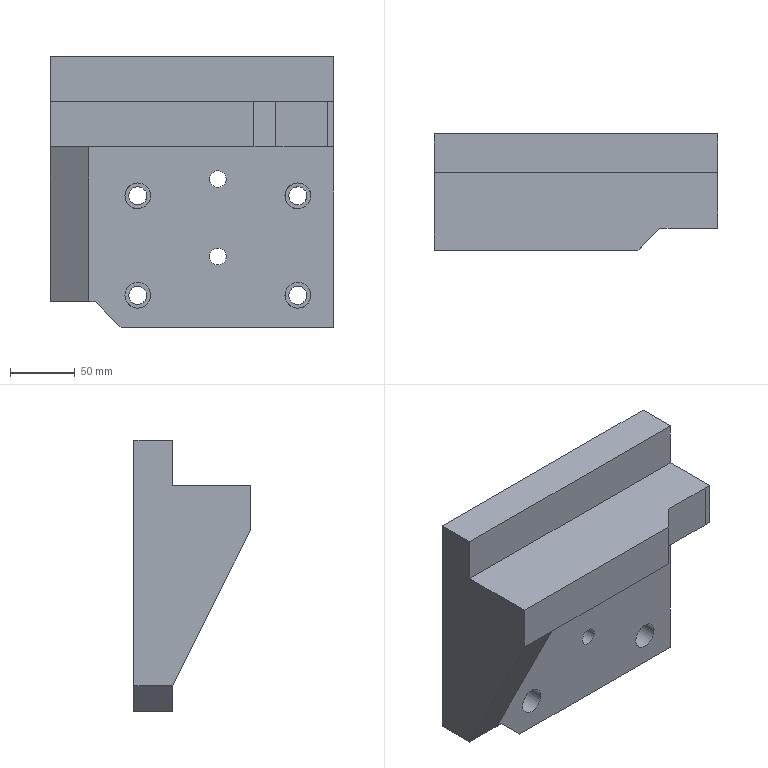Part | NX | features solid 2 | 1 solid | 31 faces | box 220 x 90 x 210 mm | volume 1861118 mm3 | plane 21 | cylinder 10 | commonest cylinder face diameters 14 x4 20 x4 13 x2
STEP:
#1=CARTESIAN_POINT('',(248.,505.,-125.));
#2=VERTEX_POINT('',#1);
#3=CARTESIAN_POINT('',(120.,505.,-125.));
#4=VERTEX_POINT('',#3);
#5=CARTESIAN_POINT('',(-235.,505.,-125.));
#6=DIRECTION('',(-1.,0.,0.));
#7=VECTOR('',#6,1000.);
#8=LINE('',#5,#7);
#9=EDGE_CURVE('',#2,#4,#8,.T.);
#10=ORIENTED_EDGE('',*,*,#9,.T.);
#11=CARTESIAN_POINT('',(120.,565.,-125.));
#12=VERTEX_POINT('',#11);
#13=CARTESIAN_POINT('',(120.,565.,-125.));
#14=DIRECTION('',(0.,1.,0.));
#15=VECTOR('',#14,1000.);
#16=LINE('',#13,#15);
#17=EDGE_CURVE('',#12,#4,#16,.F.);
#18=ORIENTED_EDGE('',*,*,#17,.F.);
#19=CARTESIAN_POINT('',(310.,565.,-125.));
#20=VERTEX_POINT('',#19);
#21=CARTESIAN_POINT('',(-235.,565.,-125.));
#22=DIRECTION('',(1.,0.,0.));
#23=VECTOR('',#22,1000.);
#24=LINE('',#21,#23);
#25=EDGE_CURVE('',#12,#20,#24,.T.);
#26=ORIENTED_EDGE('',*,*,#25,.T.);
#27=CARTESIAN_POINT('',(310.,522.,-125.));
#28=VERTEX_POINT('',#27);
#29=CARTESIAN_POINT('',(310.,565.,-125.));
#30=DIRECTION('',(0.,1.,0.));
#31=VECTOR('',#30,1000.);
#32=LINE('',#29,#31);
#33=EDGE_CURVE('',#20,#28,#32,.F.);
#34=ORIENTED_EDGE('',*,*,#33,.T.);
#35=CARTESIAN_POINT('',(305.,522.,-125.));
#36=VERTEX_POINT('',#35);
#37=CARTESIAN_POINT('',(-235.,522.,-125.));
#38=DIRECTION('',(1.,0.,0.));
#39=VECTOR('',#38,1000.);
#40=LINE('',#37,#39);
#41=EDGE_CURVE('',#28,#36,#40,.F.);
#42=ORIENTED_EDGE('',*,*,#41,.T.);
#43=CARTESIAN_POINT('',(265.,522.,-125.));
#44=VERTEX_POINT('',#43);
#45=CARTESIAN_POINT('',(-235.,522.,-125.));
#46=DIRECTION('',(1.,0.,0.));
#47=VECTOR('',#46,1000.);
#48=LINE('',#45,#47);
#49=EDGE_CURVE('',#44,#36,#48,.T.);
#50=ORIENTED_EDGE('',*,*,#49,.F.);
#51=CARTESIAN_POINT('',(36.5,293.5,-125.));
#52=DIRECTION('',(-0.7071,-0.7071,0.));
#53=VECTOR('',#52,1000.);
#54=LINE('',#51,#53);
#55=EDGE_CURVE('',#44,#2,#54,.T.);
#56=ORIENTED_EDGE('',*,*,#55,.T.);
#57=EDGE_LOOP('',(#10,#18,#26,#34,#42,#50,#56));
#58=FACE_BOUND('',#57,.T.);
#59=CARTESIAN_POINT('',(-235.,565.,-125.));
#60=DIRECTION('',(0.,0.,1.));
#61=DIRECTION('',(1.,0.,0.));
#62=AXIS2_PLACEMENT_3D('',#59,#60,#61);
#63=PLANE('',#62);
#64=ADVANCED_FACE('',(#58),#63,.F.);
#65=CARTESIAN_POINT('',(148.,565.,-163.));
#66=VERTEX_POINT('',#65);
#67=CARTESIAN_POINT('',(158.,565.,-163.));
#68=DIRECTION('',(0.,1.,0.));
#69=DIRECTION('',(-1.,0.,0.));
#70=AXIS2_PLACEMENT_3D('',#67,#68,#69);
#71=CIRCLE('',#70,10.);
#72=EDGE_CURVE('',#66,#66,#71,.F.);
#73=ORIENTED_EDGE('',*,*,#72,.F.);
#74=EDGE_LOOP('',(#73));
#75=FACE_BOUND('',#74,.T.);
#76=CARTESIAN_POINT('',(272.,565.,-163.));
#77=VERTEX_POINT('',#76);
#78=CARTESIAN_POINT('',(282.,565.,-163.));
#79=DIRECTION('',(0.,1.,0.));
#80=DIRECTION('',(-1.,0.,0.));
#81=AXIS2_PLACEMENT_3D('',#78,#79,#80);
#82=CIRCLE('',#81,10.);
#83=EDGE_CURVE('',#77,#77,#82,.F.);
#84=ORIENTED_EDGE('',*,*,#83,.F.);
#85=EDGE_LOOP('',(#84));
#86=FACE_BOUND('',#85,.T.);
#87=CARTESIAN_POINT('',(213.5,565.,-150.));
#88=VERTEX_POINT('',#87);
#89=CARTESIAN_POINT('',(220.,565.,-150.));
#90=DIRECTION('',(0.,1.,0.));
#91=DIRECTION('',(-1.,0.,0.));
#92=AXIS2_PLACEMENT_3D('',#89,#90,#91);
#93=CIRCLE('',#92,6.5);
#94=EDGE_CURVE('',#88,#88,#93,.T.);
#95=ORIENTED_EDGE('',*,*,#94,.T.);
#96=EDGE_LOOP('',(#95));
#97=FACE_BOUND('',#96,.T.);
#98=CARTESIAN_POINT('',(213.5,565.,-210.));
#99=VERTEX_POINT('',#98);
#100=CARTESIAN_POINT('',(220.,565.,-210.));
#101=DIRECTION('',(0.,1.,0.));
#102=DIRECTION('',(-1.,0.,0.));
#103=AXIS2_PLACEMENT_3D('',#100,#101,#102);
#104=CIRCLE('',#103,6.5);
#105=EDGE_CURVE('',#99,#99,#104,.T.);
#106=ORIENTED_EDGE('',*,*,#105,.T.);
#107=EDGE_LOOP('',(#106));
#108=FACE_BOUND('',#107,.T.);
#109=CARTESIAN_POINT('',(148.,565.,-240.));
#110=VERTEX_POINT('',#109);
#111=CARTESIAN_POINT('',(158.,565.,-240.));
#112=DIRECTION('',(0.,1.,0.));
#113=DIRECTION('',(-1.,0.,0.));
#114=AXIS2_PLACEMENT_3D('',#111,#112,#113);
#115=CIRCLE('',#114,10.);
#116=EDGE_CURVE('',#110,#110,#115,.F.);
#117=ORIENTED_EDGE('',*,*,#116,.F.);
#118=EDGE_LOOP('',(#117));
#119=FACE_BOUND('',#118,.T.);
#120=CARTESIAN_POINT('',(272.,565.,-240.));
#121=VERTEX_POINT('',#120);
#122=CARTESIAN_POINT('',(282.,565.,-240.));
#123=DIRECTION('',(0.,1.,0.));
#124=DIRECTION('',(-1.,0.,0.));
#125=AXIS2_PLACEMENT_3D('',#122,#123,#124);
#126=CIRCLE('',#125,10.);
#127=EDGE_CURVE('',#121,#121,#126,.F.);
#128=ORIENTED_EDGE('',*,*,#127,.F.);
#129=EDGE_LOOP('',(#128));
#130=FACE_BOUND('',#129,.T.);
#131=ORIENTED_EDGE('',*,*,#25,.F.);
#132=CARTESIAN_POINT('',(120.,565.,-245.));
#133=VERTEX_POINT('',#132);
#134=CARTESIAN_POINT('',(120.,565.,-125.));
#135=DIRECTION('',(0.,0.,-1.));
#136=VECTOR('',#135,1000.);
#137=LINE('',#134,#136);
#138=EDGE_CURVE('',#12,#133,#137,.T.);
#139=ORIENTED_EDGE('',*,*,#138,.T.);
#140=CARTESIAN_POINT('',(125.,565.,-245.));
#141=VERTEX_POINT('',#140);
#142=CARTESIAN_POINT('',(-195.,565.,-245.));
#143=DIRECTION('',(-1.,0.,0.));
#144=VECTOR('',#143,1000.);
#145=LINE('',#142,#144);
#146=EDGE_CURVE('',#133,#141,#145,.F.);
#147=ORIENTED_EDGE('',*,*,#146,.T.);
#148=CARTESIAN_POINT('',(145.,565.,-265.));
#149=VERTEX_POINT('',#148);
#150=CARTESIAN_POINT('',(25.487,565.,-145.487));
#151=DIRECTION('',(-0.7071,0.,0.7071));
#152=VECTOR('',#151,1000.);
#153=LINE('',#150,#152);
#154=EDGE_CURVE('',#141,#149,#153,.F.);
#155=ORIENTED_EDGE('',*,*,#154,.T.);
#156=CARTESIAN_POINT('',(310.,565.,-265.));
#157=VERTEX_POINT('',#156);
#158=CARTESIAN_POINT('',(115.,565.,-265.));
#159=DIRECTION('',(-1.,0.,0.));
#160=VECTOR('',#159,1000.);
#161=LINE('',#158,#160);
#162=EDGE_CURVE('',#149,#157,#161,.F.);
#163=ORIENTED_EDGE('',*,*,#162,.T.);
#164=CARTESIAN_POINT('',(310.,565.,-160.));
#165=DIRECTION('',(0.,0.,1.));
#166=VECTOR('',#165,1000.);
#167=LINE('',#164,#166);
#168=EDGE_CURVE('',#20,#157,#167,.F.);
#169=ORIENTED_EDGE('',*,*,#168,.F.);
#170=EDGE_LOOP('',(#131,#139,#147,#155,#163,#169));
#171=FACE_BOUND('',#170,.T.);
#172=CARTESIAN_POINT('',(115.,565.,-55.974));
#173=DIRECTION('',(0.,1.,0.));
#174=DIRECTION('',(-1.,0.,0.));
#175=AXIS2_PLACEMENT_3D('',#172,#173,#174);
#176=PLANE('',#175);
#177=ADVANCED_FACE('',(#75,#86,#97,#108,#119,#130,#171),#176,.F.);
#178=CARTESIAN_POINT('',(90.,565.,-245.));
#179=VERTEX_POINT('',#178);
#180=CARTESIAN_POINT('',(-195.,565.,-245.));
#181=DIRECTION('',(-1.,0.,0.));
#182=VECTOR('',#181,1000.);
#183=LINE('',#180,#182);
#184=EDGE_CURVE('',#179,#133,#183,.F.);
#185=ORIENTED_EDGE('',*,*,#184,.F.);
#186=CARTESIAN_POINT('',(90.,595.,-245.));
#187=VERTEX_POINT('',#186);
#188=CARTESIAN_POINT('',(90.,595.,-245.));
#189=DIRECTION('',(0.,1.,0.));
#190=VECTOR('',#189,1000.);
#191=LINE('',#188,#190);
#192=EDGE_CURVE('',#179,#187,#191,.T.);
#193=ORIENTED_EDGE('',*,*,#192,.T.);
#194=CARTESIAN_POINT('',(125.,595.,-245.));
#195=VERTEX_POINT('',#194);
#196=CARTESIAN_POINT('',(-195.,595.,-245.));
#197=DIRECTION('',(-1.,0.,0.));
#198=VECTOR('',#197,1000.);
#199=LINE('',#196,#198);
#200=EDGE_CURVE('',#187,#195,#199,.F.);
#201=ORIENTED_EDGE('',*,*,#200,.T.);
#202=CARTESIAN_POINT('',(125.,595.,-245.));
#203=DIRECTION('',(0.,-1.,0.));
#204=VECTOR('',#203,1000.);
#205=LINE('',#202,#204);
#206=EDGE_CURVE('',#195,#141,#205,.T.);
#207=ORIENTED_EDGE('',*,*,#206,.T.);
#208=ORIENTED_EDGE('',*,*,#146,.F.);
#209=EDGE_LOOP('',(#185,#193,#201,#207,#208));
#210=FACE_BOUND('',#209,.T.);
#211=CARTESIAN_POINT('',(-195.,595.,-245.));
#212=DIRECTION('',(0.,0.,-1.));
#213=DIRECTION('',(0.,-1.,0.));
#214=AXIS2_PLACEMENT_3D('',#211,#212,#213);
#215=PLANE('',#214);
#216=ADVANCED_FACE('',(#210),#215,.T.);
#217=CARTESIAN_POINT('',(151.,595.,-163.));
#218=VERTEX_POINT('',#217);
#219=CARTESIAN_POINT('',(158.,595.,-163.));
#220=DIRECTION('',(0.,1.,0.));
#221=DIRECTION('',(-1.,0.,0.));
#222=AXIS2_PLACEMENT_3D('',#219,#220,#221);
#223=CIRCLE('',#222,7.);
#224=EDGE_CURVE('',#218,#218,#223,.F.);
#225=ORIENTED_EDGE('',*,*,#224,.T.);
#226=EDGE_LOOP('',(#225));
#227=FACE_BOUND('',#226,.T.);
#228=CARTESIAN_POINT('',(275.,595.,-163.));
#229=VERTEX_POINT('',#228);
#230=CARTESIAN_POINT('',(282.,595.,-163.));
#231=DIRECTION('',(0.,1.,0.));
#232=DIRECTION('',(-1.,0.,0.));
#233=AXIS2_PLACEMENT_3D('',#230,#231,#232);
#234=CIRCLE('',#233,7.);
#235=EDGE_CURVE('',#229,#229,#234,.F.);
#236=ORIENTED_EDGE('',*,*,#235,.T.);
#237=EDGE_LOOP('',(#236));
#238=FACE_BOUND('',#237,.T.);
#239=CARTESIAN_POINT('',(213.5,595.,-150.));
#240=VERTEX_POINT('',#239);
#241=CARTESIAN_POINT('',(220.,595.,-150.));
#242=DIRECTION('',(0.,1.,0.));
#243=DIRECTION('',(-1.,0.,0.));
#244=AXIS2_PLACEMENT_3D('',#241,#242,#243);
#245=CIRCLE('',#244,6.5);
#246=EDGE_CURVE('',#240,#240,#245,.T.);
#247=ORIENTED_EDGE('',*,*,#246,.F.);
#248=EDGE_LOOP('',(#247));
#249=FACE_BOUND('',#248,.T.);
#250=CARTESIAN_POINT('',(213.5,595.,-210.));
#251=VERTEX_POINT('',#250);
#252=CARTESIAN_POINT('',(220.,595.,-210.));
#253=DIRECTION('',(0.,1.,0.));
#254=DIRECTION('',(-1.,0.,0.));
#255=AXIS2_PLACEMENT_3D('',#252,#253,#254);
#256=CIRCLE('',#255,6.5);
#257=EDGE_CURVE('',#251,#251,#256,.T.);
#258=ORIENTED_EDGE('',*,*,#257,.F.);
#259=EDGE_LOOP('',(#258));
#260=FACE_BOUND('',#259,.T.);
#261=CARTESIAN_POINT('',(151.,595.,-240.));
#262=VERTEX_POINT('',#261);
#263=CARTESIAN_POINT('',(158.,595.,-240.));
#264=DIRECTION('',(0.,1.,0.));
#265=DIRECTION('',(-1.,0.,0.));
#266=AXIS2_PLACEMENT_3D('',#263,#264,#265);
#267=CIRCLE('',#266,7.);
#268=EDGE_CURVE('',#262,#262,#267,.F.);
#269=ORIENTED_EDGE('',*,*,#268,.T.);
#270=EDGE_LOOP('',(#269));
#271=FACE_BOUND('',#270,.T.);
#272=CARTESIAN_POINT('',(275.,595.,-240.));
#273=VERTEX_POINT('',#272);
#274=CARTESIAN_POINT('',(282.,595.,-240.));
#275=DIRECTION('',(0.,1.,0.));
#276=DIRECTION('',(-1.,0.,0.));
#277=AXIS2_PLACEMENT_3D('',#274,#275,#276);
#278=CIRCLE('',#277,7.);
#279=EDGE_CURVE('',#273,#273,#278,.F.);
#280=ORIENTED_EDGE('',*,*,#279,.T.);
#281=EDGE_LOOP('',(#280));
#282=FACE_BOUND('',#281,.T.);
#283=ORIENTED_EDGE('',*,*,#200,.F.);
#284=CARTESIAN_POINT('',(90.,595.,-55.));
#285=VERTEX_POINT('',#284);
#286=CARTESIAN_POINT('',(90.,595.,-55.974));
#287=DIRECTION('',(0.,0.,1.));
#288=VECTOR('',#287,1000.);
#289=LINE('',#286,#288);
#290=EDGE_CURVE('',#187,#285,#289,.T.);
#291=ORIENTED_EDGE('',*,*,#290,.T.);
#292=CARTESIAN_POINT('',(310.,595.,-55.));
#293=VERTEX_POINT('',#292);
#294=CARTESIAN_POINT('',(-70.,595.,-55.));
#295=DIRECTION('',(-1.,0.,0.));
#296=VECTOR('',#295,1000.);
#297=LINE('',#294,#296);
#298=EDGE_CURVE('',#285,#293,#297,.F.);
#299=ORIENTED_EDGE('',*,*,#298,.T.);
#300=CARTESIAN_POINT('',(310.,595.,-265.));
#301=VERTEX_POINT('',#300);
#302=CARTESIAN_POINT('',(310.,595.,-160.));
#303=DIRECTION('',(0.,0.,1.));
#304=VECTOR('',#303,1000.);
#305=LINE('',#302,#304);
#306=EDGE_CURVE('',#293,#301,#305,.F.);
#307=ORIENTED_EDGE('',*,*,#306,.T.);
#308=CARTESIAN_POINT('',(145.,595.,-265.));
#309=VERTEX_POINT('',#308);
#310=CARTESIAN_POINT('',(115.,595.,-265.));
#311=DIRECTION('',(-1.,0.,0.));
#312=VECTOR('',#311,1000.);
#313=LINE('',#310,#312);
#314=EDGE_CURVE('',#309,#301,#313,.F.);
#315=ORIENTED_EDGE('',*,*,#314,.F.);
#316=CARTESIAN_POINT('',(125.,595.,-245.));
#317=DIRECTION('',(0.7071,0.,-0.7071));
#318=VECTOR('',#317,1000.);
#319=LINE('',#316,#318);
#320=EDGE_CURVE('',#309,#195,#319,.F.);
#321=ORIENTED_EDGE('',*,*,#320,.T.);
#322=EDGE_LOOP('',(#283,#291,#299,#307,#315,#321));
#323=FACE_BOUND('',#322,.T.);
#324=CARTESIAN_POINT('',(115.,595.,-55.974));
#325=DIRECTION('',(0.,1.,0.));
#326=DIRECTION('',(-1.,0.,0.));
#327=AXIS2_PLACEMENT_3D('',#324,#325,#326);
#328=PLANE('',#327);
#329=ADVANCED_FACE('',(#227,#238,#249,#260,#271,#282,#323),#328,.T.);
#330=CARTESIAN_POINT('',(90.,505.,-90.));
#331=VERTEX_POINT('',#330);
#332=CARTESIAN_POINT('',(90.,505.,-125.));
#333=VERTEX_POINT('',#332);
#334=CARTESIAN_POINT('',(90.,505.,-90.));
#335=DIRECTION('',(0.,0.,-1.));
#336=VECTOR('',#335,1000.);
#337=LINE('',#334,#336);
#338=EDGE_CURVE('',#331,#333,#337,.T.);
#339=ORIENTED_EDGE('',*,*,#338,.T.);
#340=CARTESIAN_POINT('',(90.,505.,-125.));
#341=DIRECTION('',(-1.,0.,0.));
#342=VECTOR('',#341,1000.);
#343=LINE('',#340,#342);
#344=EDGE_CURVE('',#333,#4,#343,.F.);
#345=ORIENTED_EDGE('',*,*,#344,.T.);
#346=ORIENTED_EDGE('',*,*,#9,.F.);
#347=CARTESIAN_POINT('',(248.,505.,-90.));
#348=VERTEX_POINT('',#347);
#349=CARTESIAN_POINT('',(248.,505.,-95.974));
#350=DIRECTION('',(0.,0.,1.));
#351=VECTOR('',#350,1000.);
#352=LINE('',#349,#351);
#353=EDGE_CURVE('',#2,#348,#352,.T.);
#354=ORIENTED_EDGE('',*,*,#353,.T.);
#355=CARTESIAN_POINT('',(-235.,505.,-90.));
#356=DIRECTION('',(-1.,0.,0.));
#357=VECTOR('',#356,1000.);
#358=LINE('',#355,#357);
#359=EDGE_CURVE('',#331,#348,#358,.F.);
#360=ORIENTED_EDGE('',*,*,#359,.F.);
#361=EDGE_LOOP('',(#339,#345,#346,#354,#360));
#362=FACE_BOUND('',#361,.T.);
#363=CARTESIAN_POINT('',(115.,505.,-95.974));
#364=DIRECTION('',(0.,1.,0.));
#365=DIRECTION('',(-1.,0.,0.));
#366=AXIS2_PLACEMENT_3D('',#363,#364,#365);
#367=PLANE('',#366);
#368=ADVANCED_FACE('',(#362),#367,.F.);
#369=CARTESIAN_POINT('',(158.,580.,-153.));
#370=VERTEX_POINT('',#369);
#371=CARTESIAN_POINT('',(158.,580.,-163.));
#372=DIRECTION('',(0.,-1.,0.));
#373=DIRECTION('',(0.,0.,1.));
#374=AXIS2_PLACEMENT_3D('',#371,#372,#373);
#375=CIRCLE('',#374,10.);
#376=EDGE_CURVE('',#370,#370,#375,.T.);
#377=ORIENTED_EDGE('',*,*,#376,.T.);
#378=EDGE_LOOP('',(#377));
#379=FACE_BOUND('',#378,.T.);
#380=CARTESIAN_POINT('',(158.,580.,-170.));
#381=VERTEX_POINT('',#380);
#382=CARTESIAN_POINT('',(158.,580.,-163.));
#383=DIRECTION('',(0.,-1.,0.));
#384=DIRECTION('',(0.,0.,-1.));
#385=AXIS2_PLACEMENT_3D('',#382,#383,#384);
#386=CIRCLE('',#385,7.);
#387=EDGE_CURVE('',#381,#381,#386,.F.);
#388=ORIENTED_EDGE('',*,*,#387,.T.);
#389=EDGE_LOOP('',(#388));
#390=FACE_BOUND('',#389,.T.);
#391=CARTESIAN_POINT('',(158.,580.,-163.));
#392=DIRECTION('',(0.,-1.,0.));
#393=DIRECTION('',(0.,0.,-1.));
#394=AXIS2_PLACEMENT_3D('',#391,#392,#393);
#395=PLANE('',#394);
#396=ADVANCED_FACE('',(#379,#390),#395,.T.);
#397=CARTESIAN_POINT('',(282.,580.,-153.));
#398=VERTEX_POINT('',#397);
#399=CARTESIAN_POINT('',(282.,580.,-163.));
#400=DIRECTION('',(0.,-1.,0.));
#401=DIRECTION('',(0.,0.,1.));
#402=AXIS2_PLACEMENT_3D('',#399,#400,#401);
#403=CIRCLE('',#402,10.);
#404=EDGE_CURVE('',#398,#398,#403,.T.);
#405=ORIENTED_EDGE('',*,*,#404,.T.);
#406=EDGE_LOOP('',(#405));
#407=FACE_BOUND('',#406,.T.);
#408=CARTESIAN_POINT('',(282.,580.,-170.));
#409=VERTEX_POINT('',#408);
#410=CARTESIAN_POINT('',(282.,580.,-163.));
#411=DIRECTION('',(0.,-1.,0.));
#412=DIRECTION('',(0.,0.,-1.));
#413=AXIS2_PLACEMENT_3D('',#410,#411,#412);
#414=CIRCLE('',#413,7.);
#415=EDGE_CURVE('',#409,#409,#414,.F.);
#416=ORIENTED_EDGE('',*,*,#415,.T.);
#417=EDGE_LOOP('',(#416));
#418=FACE_BOUND('',#417,.T.);
#419=CARTESIAN_POINT('',(282.,580.,-163.));
#420=DIRECTION('',(0.,-1.,0.));
#421=DIRECTION('',(0.,0.,-1.));
#422=AXIS2_PLACEMENT_3D('',#419,#420,#421);
#423=PLANE('',#422);
#424=ADVANCED_FACE('',(#407,#418),#423,.T.);
#425=CARTESIAN_POINT('',(158.,580.,-230.));
#426=VERTEX_POINT('',#425);
#427=CARTESIAN_POINT('',(158.,580.,-240.));
#428=DIRECTION('',(0.,-1.,0.));
#429=DIRECTION('',(0.,0.,1.));
#430=AXIS2_PLACEMENT_3D('',#427,#428,#429);
#431=CIRCLE('',#430,10.);
#432=EDGE_CURVE('',#426,#426,#431,.T.);
#433=ORIENTED_EDGE('',*,*,#432,.T.);
#434=EDGE_LOOP('',(#433));
#435=FACE_BOUND('',#434,.T.);
#436=CARTESIAN_POINT('',(158.,580.,-247.));
#437=VERTEX_POINT('',#436);
#438=CARTESIAN_POINT('',(158.,580.,-240.));
#439=DIRECTION('',(0.,-1.,0.));
#440=DIRECTION('',(0.,0.,-1.));
#441=AXIS2_PLACEMENT_3D('',#438,#439,#440);
#442=CIRCLE('',#441,7.);
#443=EDGE_CURVE('',#437,#437,#442,.F.);
#444=ORIENTED_EDGE('',*,*,#443,.T.);
#445=EDGE_LOOP('',(#444));
#446=FACE_BOUND('',#445,.T.);
#447=CARTESIAN_POINT('',(158.,580.,-240.));
#448=DIRECTION('',(0.,-1.,0.));
#449=DIRECTION('',(0.,0.,-1.));
#450=AXIS2_PLACEMENT_3D('',#447,#448,#449);
#451=PLANE('',#450);
#452=ADVANCED_FACE('',(#435,#446),#451,.T.);
#453=CARTESIAN_POINT('',(282.,580.,-230.));
#454=VERTEX_POINT('',#453);
#455=CARTESIAN_POINT('',(282.,580.,-240.));
#456=DIRECTION('',(0.,-1.,0.));
#457=DIRECTION('',(0.,0.,1.));
#458=AXIS2_PLACEMENT_3D('',#455,#456,#457);
#459=CIRCLE('',#458,10.);
#460=EDGE_CURVE('',#454,#454,#459,.T.);
#461=ORIENTED_EDGE('',*,*,#460,.T.);
#462=EDGE_LOOP('',(#461));
#463=FACE_BOUND('',#462,.T.);
#464=CARTESIAN_POINT('',(282.,580.,-247.));
#465=VERTEX_POINT('',#464);
#466=CARTESIAN_POINT('',(282.,580.,-240.));
#467=DIRECTION('',(0.,-1.,0.));
#468=DIRECTION('',(0.,0.,-1.));
#469=AXIS2_PLACEMENT_3D('',#466,#467,#468);
#470=CIRCLE('',#469,7.);
#471=EDGE_CURVE('',#465,#465,#470,.F.);
#472=ORIENTED_EDGE('',*,*,#471,.T.);
#473=EDGE_LOOP('',(#472));
#474=FACE_BOUND('',#473,.T.);
#475=CARTESIAN_POINT('',(282.,580.,-240.));
#476=DIRECTION('',(0.,-1.,0.));
#477=DIRECTION('',(0.,0.,-1.));
#478=AXIS2_PLACEMENT_3D('',#475,#476,#477);
#479=PLANE('',#478);
#480=ADVANCED_FACE('',(#463,#474),#479,.T.);
#481=CARTESIAN_POINT('',(90.,565.,-55.));
#482=VERTEX_POINT('',#481);
#483=CARTESIAN_POINT('',(310.,565.,-55.));
#484=VERTEX_POINT('',#483);
#485=CARTESIAN_POINT('',(-70.,565.,-55.));
#486=DIRECTION('',(-1.,0.,0.));
#487=VECTOR('',#486,1000.);
#488=LINE('',#485,#487);
#489=EDGE_CURVE('',#482,#484,#488,.F.);
#490=ORIENTED_EDGE('',*,*,#489,.F.);
#491=CARTESIAN_POINT('',(90.,565.,-90.));
#492=VERTEX_POINT('',#491);
#493=CARTESIAN_POINT('',(90.,565.,-100.));
#494=DIRECTION('',(0.,0.,1.));
#495=VECTOR('',#494,1000.);
#496=LINE('',#493,#495);
#497=EDGE_CURVE('',#492,#482,#496,.T.);
#498=ORIENTED_EDGE('',*,*,#497,.F.);
#499=CARTESIAN_POINT('',(310.,565.,-90.));
#500=VERTEX_POINT('',#499);
#501=CARTESIAN_POINT('',(-235.,565.,-90.));
#502=DIRECTION('',(-1.,0.,0.));
#503=VECTOR('',#502,1000.);
#504=LINE('',#501,#503);
#505=EDGE_CURVE('',#492,#500,#504,.F.);
#506=ORIENTED_EDGE('',*,*,#505,.T.);
#507=CARTESIAN_POINT('',(310.,565.,-160.));
#508=DIRECTION('',(0.,0.,1.));
#509=VECTOR('',#508,1000.);
#510=LINE('',#507,#509);
#511=EDGE_CURVE('',#484,#500,#510,.F.);
#512=ORIENTED_EDGE('',*,*,#511,.F.);
#513=EDGE_LOOP('',(#490,#498,#506,#512));
#514=FACE_BOUND('',#513,.T.);
#515=CARTESIAN_POINT('',(115.,565.,-55.974));
#516=DIRECTION('',(0.,1.,0.));
#517=DIRECTION('',(-1.,0.,0.));
#518=AXIS2_PLACEMENT_3D('',#515,#516,#517);
#519=PLANE('',#518);
#520=ADVANCED_FACE('',(#514),#519,.F.);
#521=CARTESIAN_POINT('',(305.,522.,-90.));
#522=VERTEX_POINT('',#521);
#523=CARTESIAN_POINT('',(265.,522.,-90.));
#524=VERTEX_POINT('',#523);
#525=CARTESIAN_POINT('',(-235.,522.,-90.));
#526=DIRECTION('',(1.,0.,0.));
#527=VECTOR('',#526,1000.);
#528=LINE('',#525,#527);
#529=EDGE_CURVE('',#522,#524,#528,.F.);
#530=ORIENTED_EDGE('',*,*,#529,.F.);
#531=CARTESIAN_POINT('',(310.,522.,-90.));
#532=VERTEX_POINT('',#531);
#533=CARTESIAN_POINT('',(-235.,522.,-90.));
#534=DIRECTION('',(1.,0.,0.));
#535=VECTOR('',#534,1000.);
#536=LINE('',#533,#535);
#537=EDGE_CURVE('',#522,#532,#536,.T.);
#538=ORIENTED_EDGE('',*,*,#537,.T.);
#539=CARTESIAN_POINT('',(310.,615.,-90.));
#540=DIRECTION('',(0.,-1.,0.));
#541=VECTOR('',#540,1000.);
#542=LINE('',#539,#541);
#543=EDGE_CURVE('',#500,#532,#542,.T.);
#544=ORIENTED_EDGE('',*,*,#543,.F.);
#545=ORIENTED_EDGE('',*,*,#505,.F.);
#546=CARTESIAN_POINT('',(90.,565.,-90.));
#547=DIRECTION('',(0.,1.,0.));
#548=VECTOR('',#547,1000.);
#549=LINE('',#546,#548);
#550=EDGE_CURVE('',#492,#331,#549,.F.);
#551=ORIENTED_EDGE('',*,*,#550,.T.);
#552=ORIENTED_EDGE('',*,*,#359,.T.);
#553=CARTESIAN_POINT('',(36.5,293.5,-90.));
#554=DIRECTION('',(-0.7071,-0.7071,0.));
#555=VECTOR('',#554,1000.);
#556=LINE('',#553,#555);
#557=EDGE_CURVE('',#348,#524,#556,.F.);
#558=ORIENTED_EDGE('',*,*,#557,.T.);
#559=EDGE_LOOP('',(#530,#538,#544,#545,#551,#552,#558));
#560=FACE_BOUND('',#559,.T.);
#561=CARTESIAN_POINT('',(-235.,565.,-90.));
#562=DIRECTION('',(0.,0.,1.));
#563=DIRECTION('',(1.,0.,0.));
#564=AXIS2_PLACEMENT_3D('',#561,#562,#563);
#565=PLANE('',#564);
#566=ADVANCED_FACE('',(#560),#565,.T.);
#567=ORIENTED_EDGE('',*,*,#224,.F.);
#568=EDGE_LOOP('',(#567));
#569=FACE_BOUND('',#568,.T.);
#570=ORIENTED_EDGE('',*,*,#387,.F.);
#571=EDGE_LOOP('',(#570));
#572=FACE_BOUND('',#571,.T.);
#573=CARTESIAN_POINT('',(158.,630.,-163.));
#574=DIRECTION('',(0.,-1.,0.));
#575=DIRECTION('',(0.,0.,-1.));
#576=AXIS2_PLACEMENT_3D('',#573,#574,#575);
#577=CYLINDRICAL_SURFACE('',#576,7.);
#578=ADVANCED_FACE('',(#569,#572),#577,.F.);
#579=ORIENTED_EDGE('',*,*,#235,.F.);
#580=EDGE_LOOP('',(#579));
#581=FACE_BOUND('',#580,.T.);
#582=ORIENTED_EDGE('',*,*,#415,.F.);
#583=EDGE_LOOP('',(#582));
#584=FACE_BOUND('',#583,.T.);
#585=CARTESIAN_POINT('',(282.,630.,-163.));
#586=DIRECTION('',(0.,-1.,0.));
#587=DIRECTION('',(0.,0.,-1.));
#588=AXIS2_PLACEMENT_3D('',#585,#586,#587);
#589=CYLINDRICAL_SURFACE('',#588,7.);
#590=ADVANCED_FACE('',(#581,#584),#589,.F.);
#591=ORIENTED_EDGE('',*,*,#268,.F.);
#592=EDGE_LOOP('',(#591));
#593=FACE_BOUND('',#592,.T.);
#594=ORIENTED_EDGE('',*,*,#443,.F.);
#595=EDGE_LOOP('',(#594));
#596=FACE_BOUND('',#595,.T.);
#597=CARTESIAN_POINT('',(158.,630.,-240.));
#598=DIRECTION('',(0.,-1.,0.));
#599=DIRECTION('',(0.,0.,-1.));
#600=AXIS2_PLACEMENT_3D('',#597,#598,#599);
#601=CYLINDRICAL_SURFACE('',#600,7.);
#602=ADVANCED_FACE('',(#593,#596),#601,.F.);
#603=ORIENTED_EDGE('',*,*,#279,.F.);
#604=EDGE_LOOP('',(#603));
#605=FACE_BOUND('',#604,.T.);
#606=ORIENTED_EDGE('',*,*,#471,.F.);
#607=EDGE_LOOP('',(#606));
#608=FACE_BOUND('',#607,.T.);
#609=CARTESIAN_POINT('',(282.,630.,-240.));
#610=DIRECTION('',(0.,-1.,0.));
#611=DIRECTION('',(0.,0.,-1.));
#612=AXIS2_PLACEMENT_3D('',#609,#610,#611);
#613=CYLINDRICAL_SURFACE('',#612,7.);
#614=ADVANCED_FACE('',(#605,#608),#613,.F.);
#615=CARTESIAN_POINT('',(90.,517.,-149.));
#616=DIRECTION('',(0.,0.4472,-0.8944));
#617=VECTOR('',#616,1000.);
#618=LINE('',#615,#617);
#619=EDGE_CURVE('',#333,#179,#618,.T.);
#620=ORIENTED_EDGE('',*,*,#619,.F.);
#621=ORIENTED_EDGE('',*,*,#338,.F.);
#622=ORIENTED_EDGE('',*,*,#550,.F.);
#623=ORIENTED_EDGE('',*,*,#497,.T.);
#624=CARTESIAN_POINT('',(90.,670.,-55.));
#625=DIRECTION('',(0.,1.,0.));
#626=VECTOR('',#625,1000.);
#627=LINE('',#624,#626);
#628=EDGE_CURVE('',#285,#482,#627,.F.);
#629=ORIENTED_EDGE('',*,*,#628,.F.);
#630=ORIENTED_EDGE('',*,*,#290,.F.);
#631=ORIENTED_EDGE('',*,*,#192,.F.);
#632=EDGE_LOOP('',(#620,#621,#622,#623,#629,#630,#631));
#633=FACE_BOUND('',#632,.T.);
#634=CARTESIAN_POINT('',(90.,565.,-90.));
#635=DIRECTION('',(1.,0.,0.));
#636=DIRECTION('',(0.,0.,-1.));
#637=AXIS2_PLACEMENT_3D('',#634,#635,#636);
#638=PLANE('',#637);
#639=ADVANCED_FACE('',(#633),#638,.F.);
#640=ORIENTED_EDGE('',*,*,#298,.F.);
#641=ORIENTED_EDGE('',*,*,#628,.T.);
#642=ORIENTED_EDGE('',*,*,#489,.T.);
#643=CARTESIAN_POINT('',(310.,670.,-55.));
#644=DIRECTION('',(0.,1.,0.));
#645=VECTOR('',#644,1000.);
#646=LINE('',#643,#645);
#647=EDGE_CURVE('',#484,#293,#646,.T.);
#648=ORIENTED_EDGE('',*,*,#647,.T.);
#649=EDGE_LOOP('',(#640,#641,#642,#648));
#650=FACE_BOUND('',#649,.T.);
#651=CARTESIAN_POINT('',(-70.,670.,-55.));
#652=DIRECTION('',(0.,0.,1.));
#653=DIRECTION('',(0.,-1.,0.));
#654=AXIS2_PLACEMENT_3D('',#651,#652,#653);
#655=PLANE('',#654);
#656=ADVANCED_FACE('',(#650),#655,.T.);
#657=CARTESIAN_POINT('',(145.,615.,-265.));
#658=DIRECTION('',(0.,-1.,0.));
#659=VECTOR('',#658,1000.);
#660=LINE('',#657,#659);
#661=EDGE_CURVE('',#309,#149,#660,.T.);
#662=ORIENTED_EDGE('',*,*,#661,.F.);
#663=ORIENTED_EDGE('',*,*,#314,.T.);
#664=CARTESIAN_POINT('',(310.,615.,-265.));
#665=DIRECTION('',(0.,1.,0.));
#666=VECTOR('',#665,1000.);
#667=LINE('',#664,#666);
#668=EDGE_CURVE('',#157,#301,#667,.T.);
#669=ORIENTED_EDGE('',*,*,#668,.F.);
#670=ORIENTED_EDGE('',*,*,#162,.F.);
#671=EDGE_LOOP('',(#662,#663,#669,#670));
#672=FACE_BOUND('',#671,.T.);
#673=CARTESIAN_POINT('',(-70.,595.,-265.));
#674=DIRECTION('',(0.,0.,-1.));
#675=DIRECTION('',(0.,1.,0.));
#676=AXIS2_PLACEMENT_3D('',#673,#674,#675);
#677=PLANE('',#676);
#678=ADVANCED_FACE('',(#672),#677,.T.);
#679=ORIENTED_EDGE('',*,*,#320,.F.);
#680=ORIENTED_EDGE('',*,*,#661,.T.);
#681=ORIENTED_EDGE('',*,*,#154,.F.);
#682=ORIENTED_EDGE('',*,*,#206,.F.);
#683=EDGE_LOOP('',(#679,#680,#681,#682));
#684=FACE_BOUND('',#683,.T.);
#685=CARTESIAN_POINT('',(125.,595.,-245.));
#686=DIRECTION('',(-0.7071,0.,-0.7071));
#687=DIRECTION('',(-0.7071,0.,0.7071));
#688=AXIS2_PLACEMENT_3D('',#685,#686,#687);
#689=PLANE('',#688);
#690=ADVANCED_FACE('',(#684),#689,.T.);
#691=ORIENTED_EDGE('',*,*,#376,.F.);
#692=EDGE_LOOP('',(#691));
#693=FACE_BOUND('',#692,.T.);
#694=ORIENTED_EDGE('',*,*,#72,.T.);
#695=EDGE_LOOP('',(#694));
#696=FACE_BOUND('',#695,.T.);
#697=CARTESIAN_POINT('',(158.,530.,-163.));
#698=DIRECTION('',(0.,1.,0.));
#699=DIRECTION('',(0.,0.,1.));
#700=AXIS2_PLACEMENT_3D('',#697,#698,#699);
#701=CYLINDRICAL_SURFACE('',#700,10.);
#702=ADVANCED_FACE('',(#693,#696),#701,.F.);
#703=ORIENTED_EDGE('',*,*,#404,.F.);
#704=EDGE_LOOP('',(#703));
#705=FACE_BOUND('',#704,.T.);
#706=ORIENTED_EDGE('',*,*,#83,.T.);
#707=EDGE_LOOP('',(#706));
#708=FACE_BOUND('',#707,.T.);
#709=CARTESIAN_POINT('',(282.,530.,-163.));
#710=DIRECTION('',(0.,1.,0.));
#711=DIRECTION('',(0.,0.,1.));
#712=AXIS2_PLACEMENT_3D('',#709,#710,#711);
#713=CYLINDRICAL_SURFACE('',#712,10.);
#714=ADVANCED_FACE('',(#705,#708),#713,.F.);
#715=ORIENTED_EDGE('',*,*,#246,.T.);
#716=EDGE_LOOP('',(#715));
#717=FACE_BOUND('',#716,.T.);
#718=ORIENTED_EDGE('',*,*,#94,.F.);
#719=EDGE_LOOP('',(#718));
#720=FACE_BOUND('',#719,.T.);
#721=CARTESIAN_POINT('',(220.,615.,-150.));
#722=DIRECTION('',(0.,-1.,0.));
#723=DIRECTION('',(0.,0.,-1.));
#724=AXIS2_PLACEMENT_3D('',#721,#722,#723);
#725=CYLINDRICAL_SURFACE('',#724,6.5);
#726=ADVANCED_FACE('',(#717,#720),#725,.F.);
#727=ORIENTED_EDGE('',*,*,#257,.T.);
#728=EDGE_LOOP('',(#727));
#729=FACE_BOUND('',#728,.T.);
#730=ORIENTED_EDGE('',*,*,#105,.F.);
#731=EDGE_LOOP('',(#730));
#732=FACE_BOUND('',#731,.T.);
#733=CARTESIAN_POINT('',(220.,615.,-210.));
#734=DIRECTION('',(0.,-1.,0.));
#735=DIRECTION('',(0.,0.,-1.));
#736=AXIS2_PLACEMENT_3D('',#733,#734,#735);
#737=CYLINDRICAL_SURFACE('',#736,6.5);
#738=ADVANCED_FACE('',(#729,#732),#737,.F.);
#739=ORIENTED_EDGE('',*,*,#432,.F.);
#740=EDGE_LOOP('',(#739));
#741=FACE_BOUND('',#740,.T.);
#742=ORIENTED_EDGE('',*,*,#116,.T.);
#743=EDGE_LOOP('',(#742));
#744=FACE_BOUND('',#743,.T.);
#745=CARTESIAN_POINT('',(158.,530.,-240.));
#746=DIRECTION('',(0.,1.,0.));
#747=DIRECTION('',(0.,0.,1.));
#748=AXIS2_PLACEMENT_3D('',#745,#746,#747);
#749=CYLINDRICAL_SURFACE('',#748,10.);
#750=ADVANCED_FACE('',(#741,#744),#749,.F.);
#751=ORIENTED_EDGE('',*,*,#460,.F.);
#752=EDGE_LOOP('',(#751));
#753=FACE_BOUND('',#752,.T.);
#754=ORIENTED_EDGE('',*,*,#127,.T.);
#755=EDGE_LOOP('',(#754));
#756=FACE_BOUND('',#755,.T.);
#757=CARTESIAN_POINT('',(282.,530.,-240.));
#758=DIRECTION('',(0.,1.,0.));
#759=DIRECTION('',(0.,0.,1.));
#760=AXIS2_PLACEMENT_3D('',#757,#758,#759);
#761=CYLINDRICAL_SURFACE('',#760,10.);
#762=ADVANCED_FACE('',(#753,#756),#761,.F.);
#763=CARTESIAN_POINT('',(265.,522.,-55.));
#764=DIRECTION('',(0.,0.,-1.));
#765=VECTOR('',#764,1000.);
#766=LINE('',#763,#765);
#767=EDGE_CURVE('',#524,#44,#766,.T.);
#768=ORIENTED_EDGE('',*,*,#767,.F.);
#769=ORIENTED_EDGE('',*,*,#557,.F.);
#770=ORIENTED_EDGE('',*,*,#353,.F.);
#771=ORIENTED_EDGE('',*,*,#55,.F.);
#772=EDGE_LOOP('',(#768,#769,#770,#771));
#773=FACE_BOUND('',#772,.T.);
#774=CARTESIAN_POINT('',(253.,510.,-55.));
#775=DIRECTION('',(-0.7071,0.7071,0.));
#776=DIRECTION('',(-0.7071,-0.7071,0.));
#777=AXIS2_PLACEMENT_3D('',#774,#775,#776);
#778=PLANE('',#777);
#779=ADVANCED_FACE('',(#773),#778,.F.);
#780=ORIENTED_EDGE('',*,*,#49,.T.);
#781=CARTESIAN_POINT('',(305.,522.,-55.));
#782=DIRECTION('',(0.,0.,-1.));
#783=VECTOR('',#782,1000.);
#784=LINE('',#781,#783);
#785=EDGE_CURVE('',#522,#36,#784,.T.);
#786=ORIENTED_EDGE('',*,*,#785,.F.);
#787=ORIENTED_EDGE('',*,*,#529,.T.);
#788=ORIENTED_EDGE('',*,*,#767,.T.);
#789=EDGE_LOOP('',(#780,#786,#787,#788));
#790=FACE_BOUND('',#789,.T.);
#791=CARTESIAN_POINT('',(305.,522.,-55.));
#792=DIRECTION('',(0.,-1.,0.));
#793=DIRECTION('',(0.,0.,1.));
#794=AXIS2_PLACEMENT_3D('',#791,#792,#793);
#795=PLANE('',#794);
#796=ADVANCED_FACE('',(#790),#795,.T.);
#797=CARTESIAN_POINT('',(310.,522.,-160.));
#798=DIRECTION('',(0.,0.,-1.));
#799=VECTOR('',#798,1000.);
#800=LINE('',#797,#799);
#801=EDGE_CURVE('',#532,#28,#800,.T.);
#802=ORIENTED_EDGE('',*,*,#801,.F.);
#803=ORIENTED_EDGE('',*,*,#537,.F.);
#804=ORIENTED_EDGE('',*,*,#785,.T.);
#805=ORIENTED_EDGE('',*,*,#41,.F.);
#806=EDGE_LOOP('',(#802,#803,#804,#805));
#807=FACE_BOUND('',#806,.T.);
#808=CARTESIAN_POINT('',(305.,522.,-55.));
#809=DIRECTION('',(0.,-1.,0.));
#810=DIRECTION('',(0.,0.,1.));
#811=AXIS2_PLACEMENT_3D('',#808,#809,#810);
#812=PLANE('',#811);
#813=ADVANCED_FACE('',(#807),#812,.T.);
#814=ORIENTED_EDGE('',*,*,#543,.T.);
#815=ORIENTED_EDGE('',*,*,#801,.T.);
#816=ORIENTED_EDGE('',*,*,#33,.F.);
#817=ORIENTED_EDGE('',*,*,#168,.T.);
#818=ORIENTED_EDGE('',*,*,#668,.T.);
#819=ORIENTED_EDGE('',*,*,#306,.F.);
#820=ORIENTED_EDGE('',*,*,#647,.F.);
#821=ORIENTED_EDGE('',*,*,#511,.T.);
#822=EDGE_LOOP('',(#814,#815,#816,#817,#818,#819,#820,#821));
#823=FACE_BOUND('',#822,.T.);
#824=CARTESIAN_POINT('',(310.,615.,-160.));
#825=DIRECTION('',(1.,0.,0.));
#826=DIRECTION('',(0.,0.,-1.));
#827=AXIS2_PLACEMENT_3D('',#824,#825,#826);
#828=PLANE('',#827);
#829=ADVANCED_FACE('',(#823),#828,.T.);
#830=ORIENTED_EDGE('',*,*,#17,.T.);
#831=CARTESIAN_POINT('',(120.,517.,-149.));
#832=DIRECTION('',(0.,0.4472,-0.8944));
#833=VECTOR('',#832,1000.);
#834=LINE('',#831,#833);
#835=EDGE_CURVE('',#4,#133,#834,.T.);
#836=ORIENTED_EDGE('',*,*,#835,.T.);
#837=ORIENTED_EDGE('',*,*,#138,.F.);
#838=EDGE_LOOP('',(#830,#836,#837));
#839=FACE_BOUND('',#838,.T.);
#840=CARTESIAN_POINT('',(120.,565.,-125.));
#841=DIRECTION('',(1.,0.,0.));
#842=DIRECTION('',(0.,0.,-1.));
#843=AXIS2_PLACEMENT_3D('',#840,#841,#842);
#844=PLANE('',#843);
#845=ADVANCED_FACE('',(#839),#844,.T.);
#846=ORIENTED_EDGE('',*,*,#835,.F.);
#847=ORIENTED_EDGE('',*,*,#344,.F.);
#848=ORIENTED_EDGE('',*,*,#619,.T.);
#849=ORIENTED_EDGE('',*,*,#184,.T.);
#850=EDGE_LOOP('',(#846,#847,#848,#849));
#851=FACE_BOUND('',#850,.T.);
#852=CARTESIAN_POINT('',(90.,565.,-245.));
#853=DIRECTION('',(0.,-0.8944,-0.4472));
#854=DIRECTION('',(0.,0.4472,-0.8944));
#855=AXIS2_PLACEMENT_3D('',#852,#853,#854);
#856=PLANE('',#855);
#857=ADVANCED_FACE('',(#851),#856,.T.);
#858=CLOSED_SHELL('',(#64,#177,#216,#329,#368,#396,#424,#452,#480,#520,#566,#578,#590,#602,#614,#639,#656,#678,#690,#702,#714,#726,#738,#750,#762,#779,#796,#813,#829,#845,#857));
#859=MANIFOLD_SOLID_BREP('',#858);
#860=(LENGTH_UNIT()NAMED_UNIT(*)SI_UNIT(.MILLI.,.METRE.));
#861=UNCERTAINTY_MEASURE_WITH_UNIT(LENGTH_MEASURE(0.00001),#860,'','');
#862=(NAMED_UNIT(*)PLANE_ANGLE_UNIT()SI_UNIT($,.RADIAN.));
#863=(NAMED_UNIT(*)SI_UNIT($,.STERADIAN.)SOLID_ANGLE_UNIT());
#864=(GEOMETRIC_REPRESENTATION_CONTEXT(3)GLOBAL_UNCERTAINTY_ASSIGNED_CONTEXT((#861))GLOBAL_UNIT_ASSIGNED_CONTEXT((#860,#862,#863))REPRESENTATION_CONTEXT('',''));
#865=ADVANCED_BREP_SHAPE_REPRESENTATION('',(#859),#864);